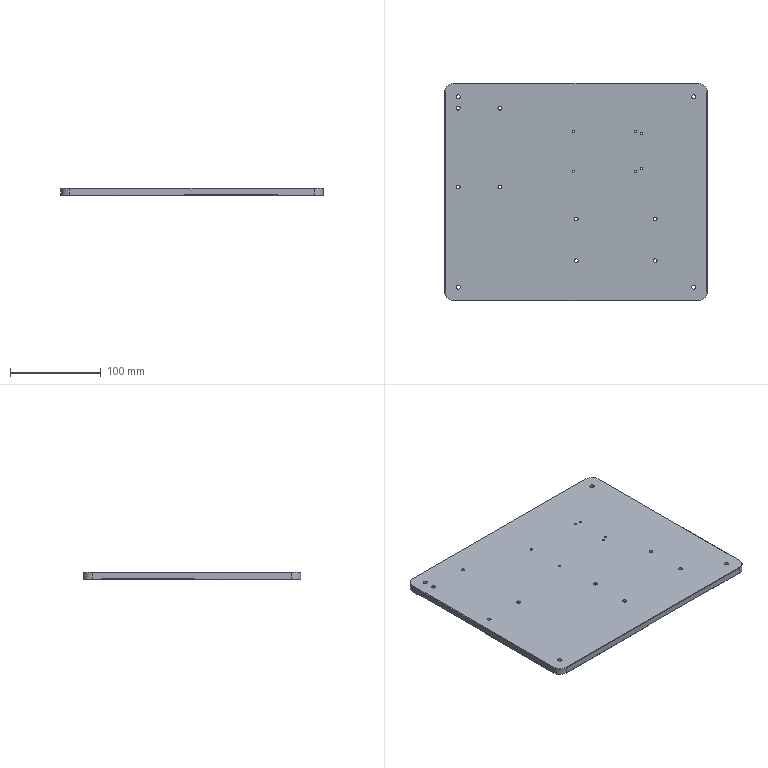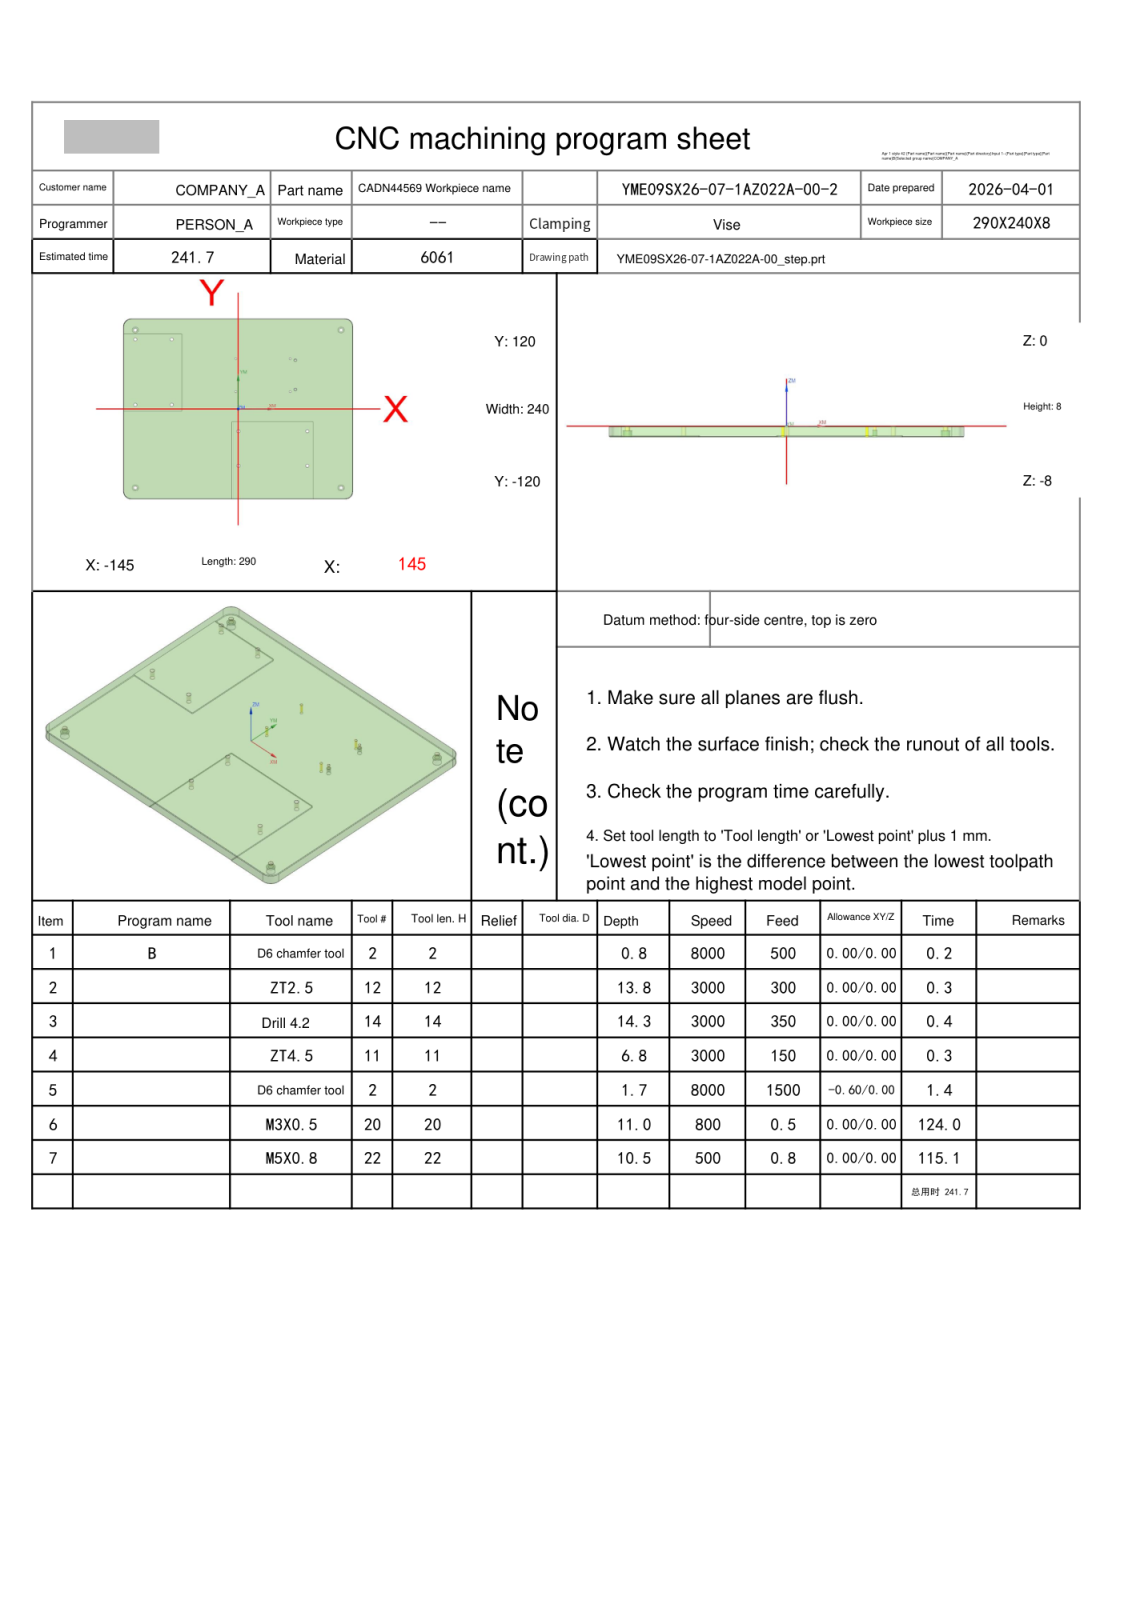NC program | NX | posted by the shop | part box 290 x 240 x 8 mm
Whole program:
%
O0001
(Machine time: 459.89 MIN)
(===Total Tool:6===)
(T2=D6 chamfer tool D=6. R=0. D- H02 Z=-1.75 )
(T12=ZT2.5  D=2.5  DR_a=118 D-  H12 Z=-13.75)
(T14=Drill 4.2 D=4.2 DR_a=118 D- H14 Z=-14.26)
(T11=ZT4.5  D=4.5  DR_a=118 D-  H11 Z=-6.75 )
(T20=M3X0.5 D=2.5  DR_a=180 D-  H20 Z=-11.  )
(T22=M5X0.8 D=4.2  DR_a=180 D-  H22 Z=-10.5 )
G80 G90 G17 G49 G40
G91 G28 Z0
M01
N1 T02 M06
(D6 chamfer tool D=6. R=0. H=02 ce=0.00 di=0.00)
G00 G90 G54 X-130. Y-105. M03 S8000
G43 H02 Z20.
M08
G98 G81 X-130. Y-105. Z-.8 R1. F500.
X-84. Y5.5
X-130.
Y92.5
Y105.
X-84. Y92.5
X-3.02 Y66.798
Y22.984
X.311 Y-29.713
Y-75.713
X87.311
X130. Y-105.
X87.311 Y-29.713
X65.705 Y22.984
X72.205 Y25.89
X65.704 Y66.798
X72.205 Y64.89
X130. Y105.
G80
G00 Z20.
G91 G28 Z0.0
M05
M09
G91 G28 Z0.0
M01
N2 T12 M06
(ZT2.5 D=2.5 DR_a=118 H=12)
G00 G90 G54 X65.705 Y22.984 M03 S3000
G43 H12 Z20.
M08
G98 G83 X65.705 Y22.984 Z-13.751 R1. F300. Q2.
G98 G83 X72.205 Y25.89 Z-8.751 R1. Q2.
Y64.89
G98 G83 X65.704 Y66.798 Z-13.751 R1. Q2.
X-3.02
Y22.984
G80
G00 Z20.
G91 G28 Z0.0
M05
M09
G91 G28 Z0.0
M01
N3 T14 M06
(Drill 4.2 D=4.2 DR_a=118 H=14)
G00 G90 G54 X-84. Y92.5 M03 S3000
G43 H14 Z20.
M08
G98 G83 X-84. Y92.5 Z-14.262 R1. F350. Q3.
X-130.
Y5.5
X-84.
X.311 Y-29.713
Y-75.713
X87.311
Y-29.713
G80
G00 Z20.
G91 G28 Z0.0
M05
M09
G91 G28 Z0.0
M01
N4 T11 M06
(ZT4.5 D=4.5 DR_a=118 H=11)
G00 G90 G54 X130. Y105. M03 S3000
G43 H11 Z20.
M08
G98 G83 X130. Y105. Z-6.752 R1. F150. Q3.
Y-105.
X-130.
Y105.
G80
G00 Z20.
G91 G28 Z0.0
M05
M09
G91 G28 Z0.0
M01
N5 T02 M06
(D6 chamfer tool D=6. R=0. H=02 ce=0.00 di=0.00)
G00 G90 G54 X65.705 Y22.984 M03 S8000
G43 H02 Z20.
M08
G98 G81 X65.705 Y22.984 Z-1.75 R3. F500.
X72.205 Y25.89
Y64.89
X65.704 Y66.798
X-3.02
Y22.984
G80
G00 Z20.
G00 G90 X-83.907 Y91.806 M03 S8000
Z20.
Z-.5
G01 Z-1. F500.
X-83.8 Y91.
G03 X-82.3 Y92.5 I0.0 J1.5
X-84. Y94.2 I-1.7 J0.0
X-85.7 Y92.5 I0.0 J-1.7
X-84. Y90.8 I1.7 J0.0
X-82.3 Y92.5 I0.0 J1.7
X-83.8 Y94. I-1.5 J0.0
G01 X-83.907 Y93.194
Z-.5
G00 Z20.
X-130.093
Z-.5
G01 Z-1.
X-130.2 Y94.
G03 X-131.7 Y92.5 I0.0 J-1.5
X-130. Y90.8 I1.7 J0.0
X-128.3 Y92.5 I0.0 J1.7
X-130. Y94.2 I-1.7 J0.0
X-131.7 Y92.5 I0.0 J-1.7
X-130.2 Y91. I1.5 J0.0
G01 X-130.093 Y91.806
Z-.5
G00 Z20.
Y6.194
Z-.5
G01 Z-1.
X-130.2 Y7.
G03 X-131.7 Y5.5 I0.0 J-1.5
X-130. Y3.8 I1.7 J0.0
X-128.3 Y5.5 I0.0 J1.7
X-130. Y7.2 I-1.7 J0.0
X-131.7 Y5.5 I0.0 J-1.7
X-130.2 Y4. I1.5 J0.0
G01 X-130.093 Y4.806
Z-.5
G00 Z20.
X-83.907
Z-.5
G01 Z-1.
X-83.8 Y4.
G03 X-82.3 Y5.5 I0.0 J1.5
X-84. Y7.2 I-1.7 J0.0
X-85.7 Y5.5 I0.0 J-1.7
X-84. Y3.8 I1.7 J0.0
X-82.3 Y5.5 I0.0 J1.7
X-83.8 Y7. I-1.5 J0.0
G01 X-83.907 Y6.194
Z-.5
G00 Z20.
X.404 Y-30.407
Z-.5
G01 Z-1.
X.511 Y-31.213
G03 X2.011 Y-29.713 I0.0 J1.5
X.311 Y-28.013 I-1.7 J0.0
X-1.389 Y-29.713 I0.0 J-1.7
X.311 Y-31.413 I1.7 J0.0
X2.011 Y-29.713 I0.0 J1.7
X.511 Y-28.213 I-1.5 J0.0
G01 X.404 Y-29.019
Z-.5
G00 Z20.
X.219 Y-75.019
Z-.5
G01 Z-1.
X.111 Y-74.213
G03 X-1.389 Y-75.713 I0.0 J-1.5
X.311 Y-77.413 I1.7 J0.0
X2.011 Y-75.713 I0.0 J1.7
X.311 Y-74.013 I-1.7 J0.0
X-1.389 Y-75.713 I0.0 J-1.7
X.111 Y-77.213 I1.5 J0.0
G01 X.219 Y-76.407
Z-.5
G00 Z20.
X87.219 Y-75.019
Z-.5
G01 Z-1.
X87.111 Y-74.213
G03 X85.611 Y-75.713 I0.0 J-1.5
X87.311 Y-77.413 I1.7 J0.0
X89.011 Y-75.713 I0.0 J1.7
X87.311 Y-74.013 I-1.7 J0.0
X85.611 Y-75.713 I0.0 J-1.7
X87.111 Y-77.213 I1.5 J0.0
G01 X87.219 Y-76.407
Z-.5
G00 Z20.
X87.404 Y-30.407
Z-.5
G01 Z-1.
X87.511 Y-31.213
G03 X89.011 Y-29.713 I0.0 J1.5
X87.311 Y-28.013 I-1.7 J0.0
X85.611 Y-29.713 I0.0 J-1.7
X87.311 Y-31.413 I1.7 J0.0
X89.011 Y-29.713 I0.0 J1.7
X87.511 Y-28.213 I-1.5 J0.0
G01 X87.404 Y-29.019
Z-.5
G00 Z20.
G00 G90 X-129.982 Y-105.55 M03 S8000
Z20.
Z-.5
G01 Z-1. F500.
X-129.95 Y-106.5
G03 X-128.45 Y-105. I0.0 J1.5
X-130. Y-103.45 I-1.55 J0.0
X-131.55 Y-105. I0.0 J-1.55
X-130. Y-106.55 I1.55 J0.0
X-128.45 Y-105. I0.0 J1.55
X-129.95 Y-103.5 I-1.5 J0.0
G01 X-129.982 Y-104.45
Z-.5
G00 Z20.
Y104.45
Z-.5
G01 Z-1.
X-129.95 Y103.5
G03 X-128.45 Y105. I0.0 J1.5
X-130. Y106.55 I-1.55 J0.0
X-131.55 Y105. I0.0 J-1.55
X-130. Y103.45 I1.55 J0.0
X-128.45 Y105. I0.0 J1.55
X-129.95 Y106.5 I-1.5 J0.0
G01 X-129.982 Y105.55
Z-.5
G00 Z20.
X130.018 Y104.45
Z-.5
G01 Z-1.
X130.05 Y103.5
G03 X131.55 Y105. I0.0 J1.5
X130. Y106.55 I-1.55 J0.0
X128.45 Y105. I0.0 J-1.55
X130. Y103.45 I1.55 J0.0
X131.55 Y105. I0.0 J1.55
X130.05 Y106.5 I-1.5 J0.0
G01 X130.018 Y105.55
Z-.5
G00 Z20.
Y-105.55
Z-.5
G01 Z-1.
X130.05 Y-106.5
G03 X131.55 Y-105. I0.0 J1.5
X130. Y-103.45 I-1.55 J0.0
X128.45 Y-105. I0.0 J-1.55
X130. Y-106.55 I1.55 J0.0
X131.55 Y-105. I0.0 J1.55
X130.05 Y-103.5 I-1.5 J0.0
G01 X130.018 Y-104.45
Z-.5
G00 Z20.
G00 G90 X136.198 Y-121.839 M03 S6500
Z20.
Z.3
G01 Z-1.2 F1500.
G03 X135. Y-120.7 I-1.198 J-.061
G01 X-135.
G02 X-145.7 Y-110. I0.0 J10.7
G01 Y110.
G02 X-145.082 Y113.583 I10.7 J0.0
X-135. Y120.7 I10.082 J-3.583
G01 X135.
G02 X145.7 Y110. I0.0 J-10.7
G01 Y-110.
G02 X135. Y-120.7 I-10.7 J0.0
G01 X134.6
G03 X133.4 Y-121.9 I0.0 J-1.2
G01 Z.3
G00 Z20.
G91 G28 Z0.0
M05
M09
G91 G28 Z0.0
M01
N6 T20 M06
(M3X0.5 D=2.5 DR_a=180 H=20)
G00 G90 G54 X65.705 Y22.984 M03 S800
G43 H20 Z20.
M08
G95
G98 G84 X65.705 Y22.984 Z-11. R1. F.5 Q5.
G98 G84 X72.205 Y25.89 Z-6. R1.
Y64.89
G98 G84 X65.704 Y66.798 Z-11. R1.
X-3.02
Y22.984
G80
G94
G00 Z20.
G91 G28 Z0.0
M05
M09
G91 G28 Z0.0
M01
N7 T22 M06
(M5X0.8 D=4.2 DR_a=180 H=22)
G00 G90 G54 X-84. Y92.5 M03 S500
G43 H22 Z20.
M08
G95
G98 G84 X-84. Y92.5 Z-10.5 R1. F.8 Q3.
X-130.
Y5.5
X-84.
X.311 Y-29.713
Y-75.713
X87.311
Y-29.713
G80
G94
G00 Z20.
M05
M09
G91 G28 Z0.0
G91 G28 Y0.0
M30
%